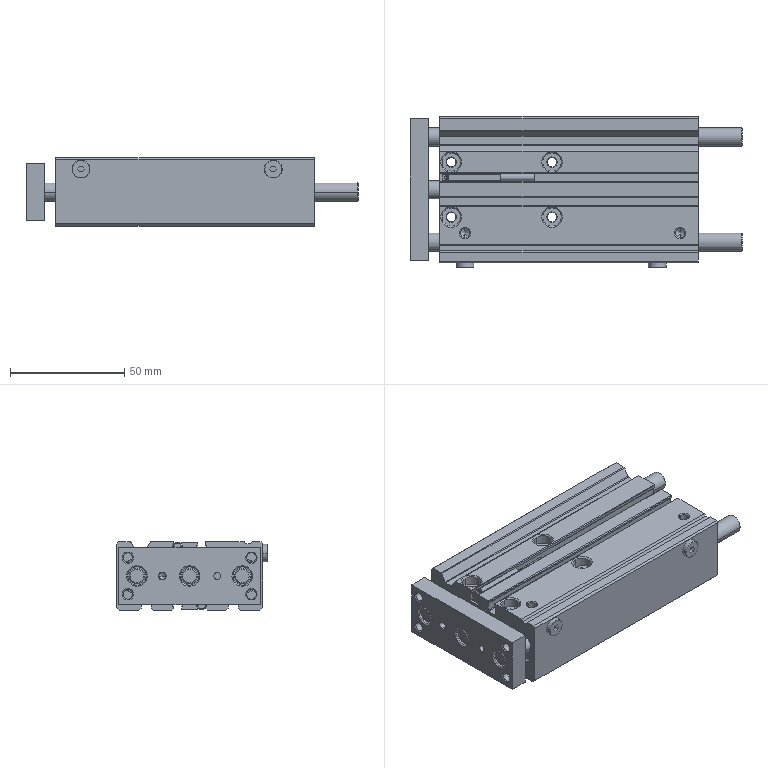Part | SolidWorks | features BaseBody 4, MoveCopyBody 1 | 4 solids | 479 faces | box 145 x 66.1 x 30 mm | volume 183701 mm3 | cylinder 189 | plane 174 | cone 114 | torus 2 | commonest cylinder face diameters 4.134 x28 8 x26 3 x25 0.4 x20 0.8 x20 0.6 x10